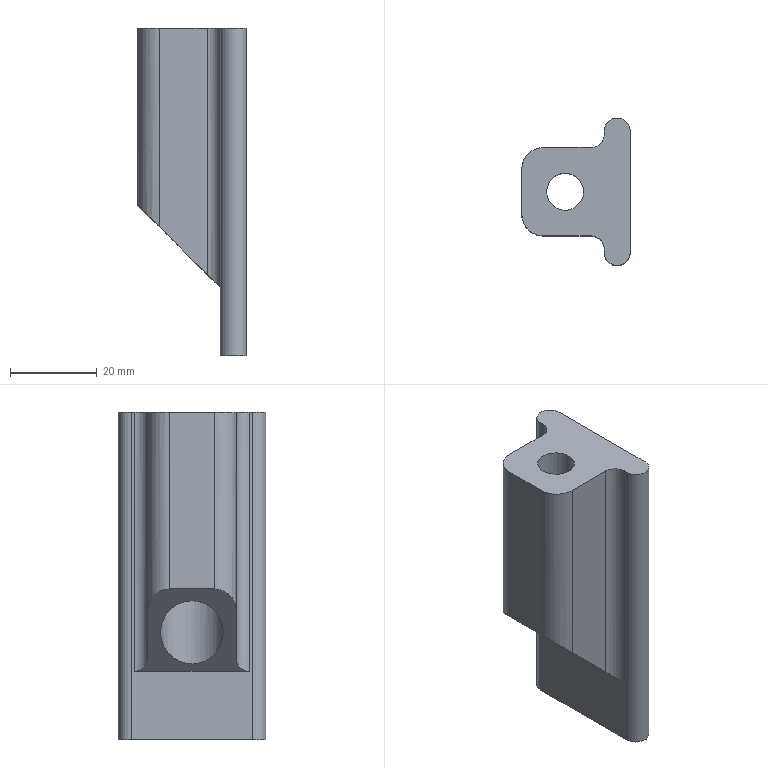Part | NX | features solid 2 | 1 solid | 17 faces | box 25 x 34 x 75.5 mm | volume 28943 mm3 | plane 9 | cylinder 8 | commonest cylinder face diameters 6 x4 10 x2 8.5 x1 14.5 x1
STEP:
#1=CARTESIAN_POINT('',(-110.306,11.898,70.));
#2=VERTEX_POINT('',#1);
#3=CARTESIAN_POINT('',(-110.306,11.098,70.));
#4=VERTEX_POINT('',#3);
#5=CARTESIAN_POINT('',(-110.306,11.898,70.));
#6=DIRECTION('',(0.,-1.,0.));
#7=VECTOR('',#6,1000.);
#8=LINE('',#5,#7);
#9=EDGE_CURVE('',#2,#4,#8,.T.);
#10=ORIENTED_EDGE('',*,*,#9,.F.);
#11=CARTESIAN_POINT('',(-110.306,11.898,-5.5));
#12=VERTEX_POINT('',#11);
#13=CARTESIAN_POINT('',(-110.306,11.898,-5.5));
#14=DIRECTION('',(0.,0.,1.));
#15=VECTOR('',#14,1000.);
#16=LINE('',#13,#15);
#17=EDGE_CURVE('',#12,#2,#16,.T.);
#18=ORIENTED_EDGE('',*,*,#17,.F.);
#19=CARTESIAN_POINT('',(-110.306,-16.102,-5.5));
#20=VERTEX_POINT('',#19);
#21=CARTESIAN_POINT('',(-110.306,-16.102,-5.5));
#22=DIRECTION('',(0.,1.,0.));
#23=VECTOR('',#22,1000.);
#24=LINE('',#21,#23);
#25=EDGE_CURVE('',#20,#12,#24,.T.);
#26=ORIENTED_EDGE('',*,*,#25,.F.);
#27=CARTESIAN_POINT('',(-110.306,-16.102,70.));
#28=VERTEX_POINT('',#27);
#29=CARTESIAN_POINT('',(-110.306,-16.102,-5.5));
#30=DIRECTION('',(0.,0.,1.));
#31=VECTOR('',#30,1000.);
#32=LINE('',#29,#31);
#33=EDGE_CURVE('',#28,#20,#32,.F.);
#34=ORIENTED_EDGE('',*,*,#33,.F.);
#35=CARTESIAN_POINT('',(-110.306,-15.302,70.));
#36=VERTEX_POINT('',#35);
#37=CARTESIAN_POINT('',(-110.306,-16.102,70.));
#38=DIRECTION('',(0.,-1.,0.));
#39=VECTOR('',#38,1000.);
#40=LINE('',#37,#39);
#41=EDGE_CURVE('',#36,#28,#40,.T.);
#42=ORIENTED_EDGE('',*,*,#41,.F.);
#43=CARTESIAN_POINT('',(-110.306,-15.302,10.261));
#44=VERTEX_POINT('',#43);
#45=CARTESIAN_POINT('',(-110.306,-15.302,-5.5));
#46=DIRECTION('',(0.,0.,-1.));
#47=VECTOR('',#46,1000.);
#48=LINE('',#45,#47);
#49=EDGE_CURVE('',#44,#36,#48,.F.);
#50=ORIENTED_EDGE('',*,*,#49,.F.);
#51=CARTESIAN_POINT('',(-110.306,11.098,10.261));
#52=VERTEX_POINT('',#51);
#53=CARTESIAN_POINT('',(-110.306,-7.302,10.261));
#54=DIRECTION('',(0.,1.,0.));
#55=VECTOR('',#54,1000.);
#56=LINE('',#53,#55);
#57=EDGE_CURVE('',#44,#52,#56,.T.);
#58=ORIENTED_EDGE('',*,*,#57,.T.);
#59=CARTESIAN_POINT('',(-110.306,11.098,-5.5));
#60=DIRECTION('',(0.,0.,-1.));
#61=VECTOR('',#60,1000.);
#62=LINE('',#59,#61);
#63=EDGE_CURVE('',#4,#52,#62,.T.);
#64=ORIENTED_EDGE('',*,*,#63,.F.);
#65=EDGE_LOOP('',(#10,#18,#26,#34,#42,#50,#58,#64));
#66=FACE_BOUND('',#65,.T.);
#67=CARTESIAN_POINT('',(-110.306,-16.102,-5.5));
#68=DIRECTION('',(-1.,0.,0.));
#69=DIRECTION('',(0.,0.,-1.));
#70=AXIS2_PLACEMENT_3D('',#67,#68,#69);
#71=PLANE('',#70);
#72=ADVANCED_FACE('',(#66),#71,.T.);
#73=CARTESIAN_POINT('',(-129.306,-7.302,70.));
#74=VERTEX_POINT('',#73);
#75=CARTESIAN_POINT('',(-129.306,3.098,70.));
#76=VERTEX_POINT('',#75);
#77=CARTESIAN_POINT('',(-129.306,-2.102,70.));
#78=DIRECTION('',(0.,-1.,0.));
#79=VECTOR('',#78,1000.);
#80=LINE('',#77,#79);
#81=EDGE_CURVE('',#74,#76,#80,.F.);
#82=ORIENTED_EDGE('',*,*,#81,.F.);
#83=CARTESIAN_POINT('',(-124.306,-12.302,70.));
#84=VERTEX_POINT('',#83);
#85=CARTESIAN_POINT('',(-124.306,-7.302,70.));
#86=DIRECTION('',(0.,0.,-1.));
#87=DIRECTION('',(-1.,0.,0.));
#88=AXIS2_PLACEMENT_3D('',#85,#86,#87);
#89=CIRCLE('',#88,5.);
#90=EDGE_CURVE('',#84,#74,#89,.T.);
#91=ORIENTED_EDGE('',*,*,#90,.F.);
#92=CARTESIAN_POINT('',(-113.306,-12.302,70.));
#93=VERTEX_POINT('',#92);
#94=CARTESIAN_POINT('',(-110.306,-12.302,70.));
#95=DIRECTION('',(1.,0.,0.));
#96=VECTOR('',#95,1000.);
#97=LINE('',#94,#96);
#98=EDGE_CURVE('',#93,#84,#97,.F.);
#99=ORIENTED_EDGE('',*,*,#98,.F.);
#100=CARTESIAN_POINT('',(-113.306,-15.302,70.));
#101=DIRECTION('',(0.,0.,-1.));
#102=DIRECTION('',(-1.,0.,0.));
#103=AXIS2_PLACEMENT_3D('',#100,#101,#102);
#104=CIRCLE('',#103,3.);
#105=EDGE_CURVE('',#36,#93,#104,.F.);
#106=ORIENTED_EDGE('',*,*,#105,.F.);
#107=ORIENTED_EDGE('',*,*,#41,.T.);
#108=CARTESIAN_POINT('',(-104.306,-16.102,70.));
#109=VERTEX_POINT('',#108);
#110=CARTESIAN_POINT('',(-107.306,-16.102,70.));
#111=DIRECTION('',(0.,0.,-1.));
#112=DIRECTION('',(-1.,0.,0.));
#113=AXIS2_PLACEMENT_3D('',#110,#111,#112);
#114=CIRCLE('',#113,3.);
#115=EDGE_CURVE('',#109,#28,#114,.T.);
#116=ORIENTED_EDGE('',*,*,#115,.F.);
#117=CARTESIAN_POINT('',(-104.306,11.898,70.));
#118=VERTEX_POINT('',#117);
#119=CARTESIAN_POINT('',(-104.306,-16.102,70.));
#120=DIRECTION('',(0.,1.,0.));
#121=VECTOR('',#120,1000.);
#122=LINE('',#119,#121);
#123=EDGE_CURVE('',#109,#118,#122,.T.);
#124=ORIENTED_EDGE('',*,*,#123,.T.);
#125=CARTESIAN_POINT('',(-107.306,11.898,70.));
#126=DIRECTION('',(0.,0.,-1.));
#127=DIRECTION('',(-1.,0.,0.));
#128=AXIS2_PLACEMENT_3D('',#125,#126,#127);
#129=CIRCLE('',#128,3.);
#130=EDGE_CURVE('',#2,#118,#129,.T.);
#131=ORIENTED_EDGE('',*,*,#130,.F.);
#132=ORIENTED_EDGE('',*,*,#9,.T.);
#133=CARTESIAN_POINT('',(-113.306,8.098,70.));
#134=VERTEX_POINT('',#133);
#135=CARTESIAN_POINT('',(-113.306,11.098,70.));
#136=DIRECTION('',(0.,0.,-1.));
#137=DIRECTION('',(-1.,0.,0.));
#138=AXIS2_PLACEMENT_3D('',#135,#136,#137);
#139=CIRCLE('',#138,3.);
#140=EDGE_CURVE('',#134,#4,#139,.F.);
#141=ORIENTED_EDGE('',*,*,#140,.F.);
#142=CARTESIAN_POINT('',(-124.306,8.098,70.));
#143=VERTEX_POINT('',#142);
#144=CARTESIAN_POINT('',(-141.111,8.098,70.));
#145=DIRECTION('',(1.,0.,0.));
#146=VECTOR('',#145,1000.);
#147=LINE('',#144,#146);
#148=EDGE_CURVE('',#134,#143,#147,.F.);
#149=ORIENTED_EDGE('',*,*,#148,.T.);
#150=CARTESIAN_POINT('',(-124.306,3.098,70.));
#151=DIRECTION('',(0.,0.,-1.));
#152=DIRECTION('',(-1.,0.,0.));
#153=AXIS2_PLACEMENT_3D('',#150,#151,#152);
#154=CIRCLE('',#153,5.);
#155=EDGE_CURVE('',#76,#143,#154,.T.);
#156=ORIENTED_EDGE('',*,*,#155,.F.);
#157=EDGE_LOOP('',(#82,#91,#99,#106,#107,#116,#124,#131,#132,#141,#149,#156));
#158=FACE_BOUND('',#157,.T.);
#159=CARTESIAN_POINT('',(-123.556,-2.102,70.));
#160=VERTEX_POINT('',#159);
#161=CARTESIAN_POINT('',(-119.306,-2.102,70.));
#162=DIRECTION('',(0.,0.,-1.));
#163=DIRECTION('',(-1.,0.,0.));
#164=AXIS2_PLACEMENT_3D('',#161,#162,#163);
#165=CIRCLE('',#164,4.25);
#166=EDGE_CURVE('',#160,#160,#165,.T.);
#167=ORIENTED_EDGE('',*,*,#166,.T.);
#168=EDGE_LOOP('',(#167));
#169=FACE_BOUND('',#168,.T.);
#170=CARTESIAN_POINT('',(-141.111,0.,70.));
#171=DIRECTION('',(0.,0.,1.));
#172=DIRECTION('',(-1.,0.,0.));
#173=AXIS2_PLACEMENT_3D('',#170,#171,#172);
#174=PLANE('',#173);
#175=ADVANCED_FACE('',(#158,#169),#174,.T.);
#176=CARTESIAN_POINT('',(-104.306,11.898,-5.5));
#177=VERTEX_POINT('',#176);
#178=CARTESIAN_POINT('',(-107.306,11.898,-5.5));
#179=DIRECTION('',(0.,0.,1.));
#180=DIRECTION('',(1.,0.,0.));
#181=AXIS2_PLACEMENT_3D('',#178,#179,#180);
#182=CIRCLE('',#181,3.);
#183=EDGE_CURVE('',#177,#12,#182,.T.);
#184=ORIENTED_EDGE('',*,*,#183,.F.);
#185=CARTESIAN_POINT('',(-104.306,-16.102,-5.5));
#186=VERTEX_POINT('',#185);
#187=CARTESIAN_POINT('',(-104.306,-16.102,-5.5));
#188=DIRECTION('',(0.,-1.,0.));
#189=VECTOR('',#188,1000.);
#190=LINE('',#187,#189);
#191=EDGE_CURVE('',#177,#186,#190,.T.);
#192=ORIENTED_EDGE('',*,*,#191,.T.);
#193=CARTESIAN_POINT('',(-107.306,-16.102,-5.5));
#194=DIRECTION('',(0.,0.,1.));
#195=DIRECTION('',(1.,0.,0.));
#196=AXIS2_PLACEMENT_3D('',#193,#194,#195);
#197=CIRCLE('',#196,3.);
#198=EDGE_CURVE('',#20,#186,#197,.T.);
#199=ORIENTED_EDGE('',*,*,#198,.F.);
#200=ORIENTED_EDGE('',*,*,#25,.T.);
#201=EDGE_LOOP('',(#184,#192,#199,#200));
#202=FACE_BOUND('',#201,.T.);
#203=CARTESIAN_POINT('',(-110.327,-2.091,-5.5));
#204=DIRECTION('',(0.,0.,1.));
#205=DIRECTION('',(-1.,0.,0.));
#206=AXIS2_PLACEMENT_3D('',#203,#204,#205);
#207=PLANE('',#206);
#208=ADVANCED_FACE('',(#202),#207,.F.);
#209=CARTESIAN_POINT('',(-124.306,8.098,24.261));
#210=VERTEX_POINT('',#209);
#211=CARTESIAN_POINT('',(-113.306,8.098,13.261));
#212=VERTEX_POINT('',#211);
#213=CARTESIAN_POINT('',(-116.425,8.098,16.381));
#214=DIRECTION('',(-0.7071,0.,0.7071));
#215=VECTOR('',#214,1000.);
#216=LINE('',#213,#215);
#217=EDGE_CURVE('',#210,#212,#216,.F.);
#218=ORIENTED_EDGE('',*,*,#217,.F.);
#219=CARTESIAN_POINT('',(-124.306,8.098,22.5));
#220=DIRECTION('',(0.,0.,-1.));
#221=VECTOR('',#220,1000.);
#222=LINE('',#219,#221);
#223=EDGE_CURVE('',#143,#210,#222,.T.);
#224=ORIENTED_EDGE('',*,*,#223,.F.);
#225=ORIENTED_EDGE('',*,*,#148,.F.);
#226=CARTESIAN_POINT('',(-113.306,8.098,22.5));
#227=DIRECTION('',(0.,0.,1.));
#228=VECTOR('',#227,1000.);
#229=LINE('',#226,#228);
#230=EDGE_CURVE('',#212,#134,#229,.T.);
#231=ORIENTED_EDGE('',*,*,#230,.F.);
#232=EDGE_LOOP('',(#218,#224,#225,#231));
#233=FACE_BOUND('',#232,.T.);
#234=CARTESIAN_POINT('',(-110.306,8.098,22.5));
#235=DIRECTION('',(0.,1.,0.));
#236=DIRECTION('',(0.,0.,1.));
#237=AXIS2_PLACEMENT_3D('',#234,#235,#236);
#238=PLANE('',#237);
#239=ADVANCED_FACE('',(#233),#238,.T.);
#240=ORIENTED_EDGE('',*,*,#98,.T.);
#241=CARTESIAN_POINT('',(-124.306,-12.302,24.261));
#242=VERTEX_POINT('',#241);
#243=CARTESIAN_POINT('',(-124.306,-12.302,22.5));
#244=DIRECTION('',(0.,0.,1.));
#245=VECTOR('',#244,1000.);
#246=LINE('',#243,#245);
#247=EDGE_CURVE('',#242,#84,#246,.T.);
#248=ORIENTED_EDGE('',*,*,#247,.F.);
#249=CARTESIAN_POINT('',(-113.306,-12.302,13.261));
#250=VERTEX_POINT('',#249);
#251=CARTESIAN_POINT('',(-116.425,-12.302,16.381));
#252=DIRECTION('',(0.7071,0.,-0.7071));
#253=VECTOR('',#252,1000.);
#254=LINE('',#251,#253);
#255=EDGE_CURVE('',#250,#242,#254,.F.);
#256=ORIENTED_EDGE('',*,*,#255,.F.);
#257=CARTESIAN_POINT('',(-113.306,-12.302,22.5));
#258=DIRECTION('',(0.,0.,1.));
#259=VECTOR('',#258,1000.);
#260=LINE('',#257,#259);
#261=EDGE_CURVE('',#93,#250,#260,.F.);
#262=ORIENTED_EDGE('',*,*,#261,.F.);
#263=EDGE_LOOP('',(#240,#248,#256,#262));
#264=FACE_BOUND('',#263,.T.);
#265=CARTESIAN_POINT('',(-110.306,-12.302,22.5));
#266=DIRECTION('',(0.,-1.,0.));
#267=DIRECTION('',(0.,0.,-1.));
#268=AXIS2_PLACEMENT_3D('',#265,#266,#267);
#269=PLANE('',#268);
#270=ADVANCED_FACE('',(#264),#269,.T.);
#271=CARTESIAN_POINT('',(-129.306,-7.302,29.261));
#272=VERTEX_POINT('',#271);
#273=CARTESIAN_POINT('',(-129.306,3.098,29.261));
#274=VERTEX_POINT('',#273);
#275=CARTESIAN_POINT('',(-129.306,-2.102,29.261));
#276=DIRECTION('',(0.,-1.,0.));
#277=VECTOR('',#276,1000.);
#278=LINE('',#275,#277);
#279=EDGE_CURVE('',#272,#274,#278,.F.);
#280=ORIENTED_EDGE('',*,*,#279,.F.);
#281=CARTESIAN_POINT('',(-129.306,-7.302,22.5));
#282=DIRECTION('',(0.,0.,1.));
#283=VECTOR('',#282,1000.);
#284=LINE('',#281,#283);
#285=EDGE_CURVE('',#74,#272,#284,.F.);
#286=ORIENTED_EDGE('',*,*,#285,.F.);
#287=ORIENTED_EDGE('',*,*,#81,.T.);
#288=CARTESIAN_POINT('',(-129.306,3.098,22.5));
#289=DIRECTION('',(0.,0.,-1.));
#290=VECTOR('',#289,1000.);
#291=LINE('',#288,#290);
#292=EDGE_CURVE('',#274,#76,#291,.F.);
#293=ORIENTED_EDGE('',*,*,#292,.F.);
#294=EDGE_LOOP('',(#280,#286,#287,#293));
#295=FACE_BOUND('',#294,.T.);
#296=CARTESIAN_POINT('',(-129.306,-2.102,22.5));
#297=DIRECTION('',(-1.,0.,0.));
#298=DIRECTION('',(0.,0.,-1.));
#299=AXIS2_PLACEMENT_3D('',#296,#297,#298);
#300=PLANE('',#299);
#301=ADVANCED_FACE('',(#295),#300,.T.);
#302=CARTESIAN_POINT('',(-126.556,-2.102,26.511));
#303=VERTEX_POINT('',#302);
#304=CARTESIAN_POINT('',(-119.306,-2.102,19.261));
#305=DIRECTION('',(-0.7071,0.,-0.7071));
#306=DIRECTION('',(-0.7071,0.,0.7071));
#307=AXIS2_PLACEMENT_3D('',#304,#305,#306);
#308=ELLIPSE('',#307,10.253,7.25);
#309=EDGE_CURVE('',#303,#303,#308,.F.);
#310=ORIENTED_EDGE('',*,*,#309,.T.);
#311=EDGE_LOOP('',(#310));
#312=FACE_BOUND('',#311,.T.);
#313=ORIENTED_EDGE('',*,*,#217,.T.);
#314=CARTESIAN_POINT('',(-113.306,11.098,13.261));
#315=DIRECTION('',(-0.7071,0.,-0.7071));
#316=DIRECTION('',(0.7071,0.,-0.7071));
#317=AXIS2_PLACEMENT_3D('',#314,#315,#316);
#318=ELLIPSE('',#317,4.243,3.);
#319=EDGE_CURVE('',#52,#212,#318,.T.);
#320=ORIENTED_EDGE('',*,*,#319,.F.);
#321=ORIENTED_EDGE('',*,*,#57,.F.);
#322=CARTESIAN_POINT('',(-113.306,-15.302,13.261));
#323=DIRECTION('',(-0.7071,0.,-0.7071));
#324=DIRECTION('',(0.7071,0.,-0.7071));
#325=AXIS2_PLACEMENT_3D('',#322,#323,#324);
#326=ELLIPSE('',#325,4.243,3.);
#327=EDGE_CURVE('',#250,#44,#326,.T.);
#328=ORIENTED_EDGE('',*,*,#327,.F.);
#329=ORIENTED_EDGE('',*,*,#255,.T.);
#330=CARTESIAN_POINT('',(-124.306,-7.302,24.261));
#331=DIRECTION('',(-0.7071,0.,-0.7071));
#332=DIRECTION('',(0.7071,0.,-0.7071));
#333=AXIS2_PLACEMENT_3D('',#330,#331,#332);
#334=ELLIPSE('',#333,7.071,5.);
#335=EDGE_CURVE('',#272,#242,#334,.F.);
#336=ORIENTED_EDGE('',*,*,#335,.F.);
#337=ORIENTED_EDGE('',*,*,#279,.T.);
#338=CARTESIAN_POINT('',(-124.306,3.098,24.261));
#339=DIRECTION('',(-0.7071,0.,-0.7071));
#340=DIRECTION('',(-0.7071,0.,0.7071));
#341=AXIS2_PLACEMENT_3D('',#338,#339,#340);
#342=ELLIPSE('',#341,7.071,5.);
#343=EDGE_CURVE('',#210,#274,#342,.F.);
#344=ORIENTED_EDGE('',*,*,#343,.F.);
#345=EDGE_LOOP('',(#313,#320,#321,#328,#329,#336,#337,#344));
#346=FACE_BOUND('',#345,.T.);
#347=CARTESIAN_POINT('',(-113.306,-7.302,13.261));
#348=DIRECTION('',(-0.7071,0.,-0.7071));
#349=DIRECTION('',(-0.7071,0.,0.7071));
#350=AXIS2_PLACEMENT_3D('',#347,#348,#349);
#351=PLANE('',#350);
#352=ADVANCED_FACE('',(#312,#346),#351,.T.);
#353=ORIENTED_EDGE('',*,*,#166,.F.);
#354=EDGE_LOOP('',(#353));
#355=FACE_BOUND('',#354,.T.);
#356=CARTESIAN_POINT('',(-123.556,-2.102,40.));
#357=VERTEX_POINT('',#356);
#358=CARTESIAN_POINT('',(-119.306,-2.102,40.));
#359=DIRECTION('',(0.,0.,-1.));
#360=DIRECTION('',(-1.,0.,0.));
#361=AXIS2_PLACEMENT_3D('',#358,#359,#360);
#362=CIRCLE('',#361,4.25);
#363=EDGE_CURVE('',#357,#357,#362,.T.);
#364=ORIENTED_EDGE('',*,*,#363,.T.);
#365=EDGE_LOOP('',(#364));
#366=FACE_BOUND('',#365,.T.);
#367=CARTESIAN_POINT('',(-119.306,-2.102,2.));
#368=DIRECTION('',(0.,0.,1.));
#369=DIRECTION('',(-1.,0.,0.));
#370=AXIS2_PLACEMENT_3D('',#367,#368,#369);
#371=CYLINDRICAL_SURFACE('',#370,4.25);
#372=ADVANCED_FACE('',(#355,#366),#371,.F.);
#373=ORIENTED_EDGE('',*,*,#363,.F.);
#374=EDGE_LOOP('',(#373));
#375=FACE_BOUND('',#374,.T.);
#376=CARTESIAN_POINT('',(-126.556,-2.102,40.));
#377=VERTEX_POINT('',#376);
#378=CARTESIAN_POINT('',(-119.306,-2.102,40.));
#379=DIRECTION('',(0.,0.,-1.));
#380=DIRECTION('',(-1.,0.,0.));
#381=AXIS2_PLACEMENT_3D('',#378,#379,#380);
#382=CIRCLE('',#381,7.25);
#383=EDGE_CURVE('',#377,#377,#382,.T.);
#384=ORIENTED_EDGE('',*,*,#383,.T.);
#385=EDGE_LOOP('',(#384));
#386=FACE_BOUND('',#385,.T.);
#387=CARTESIAN_POINT('',(-141.111,0.,40.));
#388=DIRECTION('',(0.,0.,1.));
#389=DIRECTION('',(-1.,0.,0.));
#390=AXIS2_PLACEMENT_3D('',#387,#388,#389);
#391=PLANE('',#390);
#392=ADVANCED_FACE('',(#375,#386),#391,.F.);
#393=ORIENTED_EDGE('',*,*,#309,.F.);
#394=EDGE_LOOP('',(#393));
#395=FACE_BOUND('',#394,.T.);
#396=ORIENTED_EDGE('',*,*,#383,.F.);
#397=EDGE_LOOP('',(#396));
#398=FACE_BOUND('',#397,.T.);
#399=CARTESIAN_POINT('',(-119.306,-2.102,2.));
#400=DIRECTION('',(0.,0.,1.));
#401=DIRECTION('',(-1.,0.,0.));
#402=AXIS2_PLACEMENT_3D('',#399,#400,#401);
#403=CYLINDRICAL_SURFACE('',#402,7.25);
#404=ADVANCED_FACE('',(#395,#398),#403,.F.);
#405=ORIENTED_EDGE('',*,*,#191,.F.);
#406=CARTESIAN_POINT('',(-104.306,11.898,-5.5));
#407=DIRECTION('',(0.,0.,1.));
#408=VECTOR('',#407,1000.);
#409=LINE('',#406,#408);
#410=EDGE_CURVE('',#118,#177,#409,.F.);
#411=ORIENTED_EDGE('',*,*,#410,.F.);
#412=ORIENTED_EDGE('',*,*,#123,.F.);
#413=CARTESIAN_POINT('',(-104.306,-16.102,-5.5));
#414=DIRECTION('',(0.,0.,1.));
#415=VECTOR('',#414,1000.);
#416=LINE('',#413,#415);
#417=EDGE_CURVE('',#186,#109,#416,.T.);
#418=ORIENTED_EDGE('',*,*,#417,.F.);
#419=EDGE_LOOP('',(#405,#411,#412,#418));
#420=FACE_BOUND('',#419,.T.);
#421=CARTESIAN_POINT('',(-104.306,-16.102,-5.5));
#422=DIRECTION('',(1.,0.,0.));
#423=DIRECTION('',(0.,0.,1.));
#424=AXIS2_PLACEMENT_3D('',#421,#422,#423);
#425=PLANE('',#424);
#426=ADVANCED_FACE('',(#420),#425,.T.);
#427=ORIENTED_EDGE('',*,*,#417,.T.);
#428=ORIENTED_EDGE('',*,*,#115,.T.);
#429=ORIENTED_EDGE('',*,*,#33,.T.);
#430=ORIENTED_EDGE('',*,*,#198,.T.);
#431=EDGE_LOOP('',(#427,#428,#429,#430));
#432=FACE_BOUND('',#431,.T.);
#433=CARTESIAN_POINT('',(-107.306,-16.102,-5.5));
#434=DIRECTION('',(0.,0.,1.));
#435=DIRECTION('',(-1.,0.,0.));
#436=AXIS2_PLACEMENT_3D('',#433,#434,#435);
#437=CYLINDRICAL_SURFACE('',#436,3.);
#438=ADVANCED_FACE('',(#432),#437,.T.);
#439=ORIENTED_EDGE('',*,*,#130,.T.);
#440=ORIENTED_EDGE('',*,*,#410,.T.);
#441=ORIENTED_EDGE('',*,*,#183,.T.);
#442=ORIENTED_EDGE('',*,*,#17,.T.);
#443=EDGE_LOOP('',(#439,#440,#441,#442));
#444=FACE_BOUND('',#443,.T.);
#445=CARTESIAN_POINT('',(-107.306,11.898,-5.5));
#446=DIRECTION('',(0.,0.,1.));
#447=DIRECTION('',(-1.,0.,0.));
#448=AXIS2_PLACEMENT_3D('',#445,#446,#447);
#449=CYLINDRICAL_SURFACE('',#448,3.);
#450=ADVANCED_FACE('',(#444),#449,.T.);
#451=ORIENTED_EDGE('',*,*,#343,.T.);
#452=ORIENTED_EDGE('',*,*,#292,.T.);
#453=ORIENTED_EDGE('',*,*,#155,.T.);
#454=ORIENTED_EDGE('',*,*,#223,.T.);
#455=EDGE_LOOP('',(#451,#452,#453,#454));
#456=FACE_BOUND('',#455,.T.);
#457=CARTESIAN_POINT('',(-124.306,3.098,22.5));
#458=DIRECTION('',(0.,0.,1.));
#459=DIRECTION('',(-1.,0.,0.));
#460=AXIS2_PLACEMENT_3D('',#457,#458,#459);
#461=CYLINDRICAL_SURFACE('',#460,5.);
#462=ADVANCED_FACE('',(#456),#461,.T.);
#463=ORIENTED_EDGE('',*,*,#90,.T.);
#464=ORIENTED_EDGE('',*,*,#285,.T.);
#465=ORIENTED_EDGE('',*,*,#335,.T.);
#466=ORIENTED_EDGE('',*,*,#247,.T.);
#467=EDGE_LOOP('',(#463,#464,#465,#466));
#468=FACE_BOUND('',#467,.T.);
#469=CARTESIAN_POINT('',(-124.306,-7.302,22.5));
#470=DIRECTION('',(0.,0.,-1.));
#471=DIRECTION('',(1.,0.,0.));
#472=AXIS2_PLACEMENT_3D('',#469,#470,#471);
#473=CYLINDRICAL_SURFACE('',#472,5.);
#474=ADVANCED_FACE('',(#468),#473,.T.);
#475=ORIENTED_EDGE('',*,*,#319,.T.);
#476=ORIENTED_EDGE('',*,*,#230,.T.);
#477=ORIENTED_EDGE('',*,*,#140,.T.);
#478=ORIENTED_EDGE('',*,*,#63,.T.);
#479=EDGE_LOOP('',(#475,#476,#477,#478));
#480=FACE_BOUND('',#479,.T.);
#481=CARTESIAN_POINT('',(-113.306,11.098,22.5));
#482=DIRECTION('',(0.,0.,-1.));
#483=DIRECTION('',(1.,0.,0.));
#484=AXIS2_PLACEMENT_3D('',#481,#482,#483);
#485=CYLINDRICAL_SURFACE('',#484,3.);
#486=ADVANCED_FACE('',(#480),#485,.F.);
#487=ORIENTED_EDGE('',*,*,#327,.T.);
#488=ORIENTED_EDGE('',*,*,#49,.T.);
#489=ORIENTED_EDGE('',*,*,#105,.T.);
#490=ORIENTED_EDGE('',*,*,#261,.T.);
#491=EDGE_LOOP('',(#487,#488,#489,#490));
#492=FACE_BOUND('',#491,.T.);
#493=CARTESIAN_POINT('',(-113.306,-15.302,-5.5));
#494=DIRECTION('',(0.,0.,-1.));
#495=DIRECTION('',(1.,0.,0.));
#496=AXIS2_PLACEMENT_3D('',#493,#494,#495);
#497=CYLINDRICAL_SURFACE('',#496,3.);
#498=ADVANCED_FACE('',(#492),#497,.F.);
#499=CLOSED_SHELL('',(#72,#175,#208,#239,#270,#301,#352,#372,#392,#404,#426,#438,#450,#462,#474,#486,#498));
#500=MANIFOLD_SOLID_BREP('',#499);
#501=(LENGTH_UNIT()NAMED_UNIT(*)SI_UNIT(.MILLI.,.METRE.));
#502=UNCERTAINTY_MEASURE_WITH_UNIT(LENGTH_MEASURE(0.00001),#501,'','');
#503=(NAMED_UNIT(*)PLANE_ANGLE_UNIT()SI_UNIT($,.RADIAN.));
#504=(NAMED_UNIT(*)SI_UNIT($,.STERADIAN.)SOLID_ANGLE_UNIT());
#505=(GEOMETRIC_REPRESENTATION_CONTEXT(3)GLOBAL_UNCERTAINTY_ASSIGNED_CONTEXT((#502))GLOBAL_UNIT_ASSIGNED_CONTEXT((#501,#503,#504))REPRESENTATION_CONTEXT('',''));
#506=ADVANCED_BREP_SHAPE_REPRESENTATION('',(#500),#505);